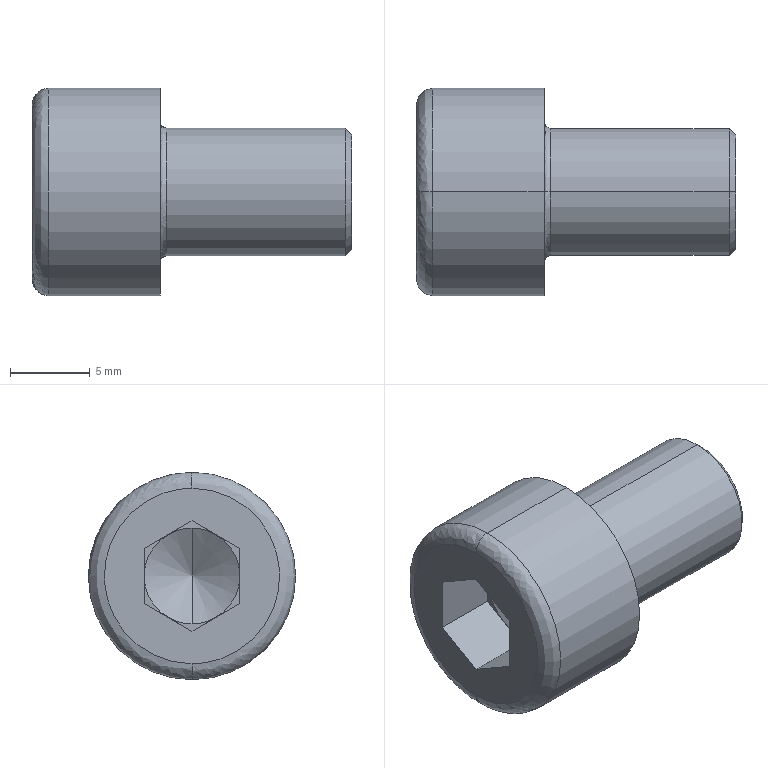Part | SolidWorks | features BaseBody 1 | 1 solid | 27 faces | box 20 x 13 x 13 mm | volume 1515 mm3 | plane 15 | spline 4 | cylinder 4 | cone 4 | commonest cylinder face diameters 8 x2 13 x2
STEP:
#1=CARTESIAN_POINT('',(1.,0.,6.5));
#2=VERTEX_POINT('',#1);
#3=CARTESIAN_POINT('',(1.,0.,-6.5));
#4=VERTEX_POINT('',#3);
#5=CARTESIAN_POINT('',(1.,0.,0.));
#6=DIRECTION('',(1.,0.,0.));
#7=DIRECTION('',(0.,0.,1.));
#8=AXIS2_PLACEMENT_3D('',#5,#6,#7);
#9=CIRCLE('',#8,6.5);
#10=EDGE_CURVE('',#2,#4,#9,.T.);
#11=ORIENTED_EDGE('',*,*,#10,.F.);
#12=CARTESIAN_POINT('',(0.,0.,5.5));
#13=VERTEX_POINT('',#12);
#14=CARTESIAN_POINT('',(1.,0.,5.5));
#15=DIRECTION('',(0.,-1.,0.));
#16=DIRECTION('',(0.,0.,1.));
#17=AXIS2_PLACEMENT_3D('',#14,#15,#16);
#18=CIRCLE('',#17,1.);
#19=EDGE_CURVE('',#2,#13,#18,.T.);
#20=ORIENTED_EDGE('',*,*,#19,.T.);
#21=CARTESIAN_POINT('',(0.,0.,-5.5));
#22=VERTEX_POINT('',#21);
#23=CARTESIAN_POINT('',(0.,0.,5.5));
#24=CARTESIAN_POINT('',(0.,-11.,5.5));
#25=CARTESIAN_POINT('',(0.,-11.,-5.5));
#26=CARTESIAN_POINT('',(0.,0.,-5.5));
#27=(BOUNDED_CURVE()B_SPLINE_CURVE(3,(#23,#24,#25,#26),.UNSPECIFIED.,.F.,.T.)B_SPLINE_CURVE_WITH_KNOTS((4,4),(0.,1.),.UNSPECIFIED.)CURVE()GEOMETRIC_REPRESENTATION_ITEM()RATIONAL_B_SPLINE_CURVE((1.,0.3333,0.3333,1.))REPRESENTATION_ITEM(''));
#28=EDGE_CURVE('',#13,#22,#27,.T.);
#29=ORIENTED_EDGE('',*,*,#28,.T.);
#30=CARTESIAN_POINT('',(1.,0.,-5.5));
#31=DIRECTION('',(0.,1.,0.));
#32=DIRECTION('',(0.,0.,-1.));
#33=AXIS2_PLACEMENT_3D('',#30,#31,#32);
#34=CIRCLE('',#33,1.);
#35=EDGE_CURVE('',#4,#22,#34,.T.);
#36=ORIENTED_EDGE('',*,*,#35,.F.);
#37=EDGE_LOOP('',(#11,#20,#29,#36));
#38=FACE_OUTER_BOUND('',#37,.T.);
#39=CARTESIAN_POINT('',(1.,0.,6.5));
#40=CARTESIAN_POINT('',(1.,-13.,6.5));
#41=CARTESIAN_POINT('',(1.,-13.,-6.5));
#42=CARTESIAN_POINT('',(1.,0.,-6.5));
#43=CARTESIAN_POINT('',(0.4142,0.,6.5));
#44=CARTESIAN_POINT('',(0.4142,-13.,6.5));
#45=CARTESIAN_POINT('',(0.4142,-13.,-6.5));
#46=CARTESIAN_POINT('',(0.4142,0.,-6.5));
#47=CARTESIAN_POINT('',(0.,0.,6.086));
#48=CARTESIAN_POINT('',(0.,-12.172,6.086));
#49=CARTESIAN_POINT('',(0.,-12.172,-6.086));
#50=CARTESIAN_POINT('',(0.,0.,-6.086));
#51=CARTESIAN_POINT('',(0.,0.,5.5));
#52=CARTESIAN_POINT('',(0.,-11.,5.5));
#53=CARTESIAN_POINT('',(0.,-11.,-5.5));
#54=CARTESIAN_POINT('',(0.,0.,-5.5));
#55=(BOUNDED_SURFACE()B_SPLINE_SURFACE(3,3,((#39,#40,#41,#42),(#43,#44,#45,#46),(#47,#48,#49,#50),(#51,#52,#53,#54)),.UNSPECIFIED.,.F.,.F.,.F.)B_SPLINE_SURFACE_WITH_KNOTS((4,4),(4,4),(0.,1.),(0.,1.),.UNSPECIFIED.)GEOMETRIC_REPRESENTATION_ITEM()RATIONAL_B_SPLINE_SURFACE(((1.,0.3333,0.3333,1.),(0.8047,0.2682,0.2682,0.8047),(0.8047,0.2682,0.2682,0.8047),(1.,0.3333,0.3333,1.)))REPRESENTATION_ITEM('')SURFACE());
#56=ADVANCED_FACE('',(#38),#55,.T.);
#57=CARTESIAN_POINT('',(8.,0.,4.4));
#58=VERTEX_POINT('',#57);
#59=CARTESIAN_POINT('',(8.,0.,-4.4));
#60=VERTEX_POINT('',#59);
#61=CARTESIAN_POINT('',(8.,0.,4.4));
#62=CARTESIAN_POINT('',(8.,0.2797,4.4));
#63=CARTESIAN_POINT('',(8.,0.6919,4.361));
#64=CARTESIAN_POINT('',(8.,1.16,4.249));
#65=CARTESIAN_POINT('',(8.,1.391,4.176));
#66=CARTESIAN_POINT('',(8.,1.489,4.141));
#67=CARTESIAN_POINT('',(8.,1.554,4.116));
#68=CARTESIAN_POINT('',(8.,1.585,4.105));
#69=CARTESIAN_POINT('',(8.,1.758,4.036));
#70=CARTESIAN_POINT('',(8.,1.96,3.944));
#71=CARTESIAN_POINT('',(8.,2.154,3.837));
#72=CARTESIAN_POINT('',(8.,2.282,3.763));
#73=CARTESIAN_POINT('',(8.,2.344,3.724));
#74=CARTESIAN_POINT('',(8.,2.662,3.517));
#75=CARTESIAN_POINT('',(8.,2.897,3.326));
#76=CARTESIAN_POINT('',(8.,3.219,3.004));
#77=CARTESIAN_POINT('',(8.,3.37,2.836));
#78=CARTESIAN_POINT('',(8.,3.509,2.656));
#79=CARTESIAN_POINT('',(8.,3.598,2.534));
#80=CARTESIAN_POINT('',(8.,3.642,2.47));
#81=CARTESIAN_POINT('',(8.,3.764,2.283));
#82=CARTESIAN_POINT('',(8.,3.876,2.092));
#83=CARTESIAN_POINT('',(8.,3.989,1.859));
#84=CARTESIAN_POINT('',(8.,4.042,1.74));
#85=CARTESIAN_POINT('',(8.,4.063,1.689));
#86=CARTESIAN_POINT('',(8.,4.077,1.654));
#87=CARTESIAN_POINT('',(8.,4.085,1.636));
#88=CARTESIAN_POINT('',(8.,4.297,1.1));
#89=CARTESIAN_POINT('',(8.,4.4,0.5592));
#90=CARTESIAN_POINT('',(8.,4.4,-0.2796));
#91=CARTESIAN_POINT('',(8.,4.361,-0.6917));
#92=CARTESIAN_POINT('',(8.,4.249,-1.16));
#93=CARTESIAN_POINT('',(8.,4.176,-1.391));
#94=CARTESIAN_POINT('',(8.,4.141,-1.489));
#95=CARTESIAN_POINT('',(8.,4.116,-1.554));
#96=CARTESIAN_POINT('',(8.,4.105,-1.585));
#97=CARTESIAN_POINT('',(8.,4.036,-1.758));
#98=CARTESIAN_POINT('',(8.,3.944,-1.96));
#99=CARTESIAN_POINT('',(8.,3.837,-2.154));
#100=CARTESIAN_POINT('',(8.,3.763,-2.282));
#101=CARTESIAN_POINT('',(8.,3.724,-2.344));
#102=CARTESIAN_POINT('',(8.,3.517,-2.662));
#103=CARTESIAN_POINT('',(8.,3.326,-2.897));
#104=CARTESIAN_POINT('',(8.,3.004,-3.219));
#105=CARTESIAN_POINT('',(8.,2.836,-3.37));
#106=CARTESIAN_POINT('',(8.,2.656,-3.509));
#107=CARTESIAN_POINT('',(8.,2.534,-3.598));
#108=CARTESIAN_POINT('',(8.,2.47,-3.642));
#109=CARTESIAN_POINT('',(8.,2.283,-3.764));
#110=CARTESIAN_POINT('',(8.,2.092,-3.876));
#111=CARTESIAN_POINT('',(8.,1.859,-3.989));
#112=CARTESIAN_POINT('',(8.,1.74,-4.042));
#113=CARTESIAN_POINT('',(8.,1.689,-4.063));
#114=CARTESIAN_POINT('',(8.,1.654,-4.077));
#115=CARTESIAN_POINT('',(8.,1.636,-4.085));
#116=CARTESIAN_POINT('',(8.,1.1,-4.297));
#117=CARTESIAN_POINT('',(8.,0.5597,-4.4));
#118=CARTESIAN_POINT('',(8.,0.,-4.4));
#119=B_SPLINE_CURVE_WITH_KNOTS('',3,(#61,#62,#63,#64,#65,#66,#67,#68,#69,#70,#71,#72,#73,#74,#75,#76,#77,#78,#79,#80,#81,#82,#83,#84,#85,#86,#87,#88,#89,#90,#91,#92,#93,#94,#95,#96,#97,#98,#99,#100,#101,#102,#103,#104,#105,#106,#107,#108,#109,#110,#111,#112,#113,#114,#115,#116,#117,#118),.UNSPECIFIED.,.F.,.F.,(4,1,1,1,2,2,1,2,2,2,1,2,2,1,1,1,2,2,2,1,1,1,2,2,1,2,2,2,1,2,2,1,1,1,2,2,4),(0.,0.0625,0.09375,0.1094,0.1172,0.125,0.1562,0.1719,0.1875,0.25,0.2812,0.2969,0.3125,0.3437,0.3594,0.3672,0.3711,0.375,0.5,0.5625,0.5937,0.6094,0.6172,0.625,0.6562,0.6719,0.6875,0.75,0.7812,0.7969,0.8125,0.8437,0.8594,0.8672,0.8711,0.875,1.),.UNSPECIFIED.);
#120=EDGE_CURVE('',#58,#60,#119,.T.);
#121=ORIENTED_EDGE('',*,*,#120,.F.);
#122=CARTESIAN_POINT('',(8.4,0.,4.));
#123=VERTEX_POINT('',#122);
#124=CARTESIAN_POINT('',(8.4,0.,4.4));
#125=DIRECTION('',(0.,-1.,0.));
#126=DIRECTION('',(0.,0.,1.));
#127=AXIS2_PLACEMENT_3D('',#124,#125,#126);
#128=CIRCLE('',#127,0.4);
#129=EDGE_CURVE('',#58,#123,#128,.T.);
#130=ORIENTED_EDGE('',*,*,#129,.T.);
#131=CARTESIAN_POINT('',(8.4,0.,-4.));
#132=VERTEX_POINT('',#131);
#133=CARTESIAN_POINT('',(8.4,0.,0.));
#134=DIRECTION('',(1.,0.,0.));
#135=DIRECTION('',(0.,0.,-1.));
#136=AXIS2_PLACEMENT_3D('',#133,#134,#135);
#137=CIRCLE('',#136,4.);
#138=EDGE_CURVE('',#132,#123,#137,.T.);
#139=ORIENTED_EDGE('',*,*,#138,.F.);
#140=CARTESIAN_POINT('',(8.4,0.,-4.4));
#141=DIRECTION('',(0.,1.,0.));
#142=DIRECTION('',(0.,0.,-1.));
#143=AXIS2_PLACEMENT_3D('',#140,#141,#142);
#144=CIRCLE('',#143,0.4);
#145=EDGE_CURVE('',#60,#132,#144,.T.);
#146=ORIENTED_EDGE('',*,*,#145,.F.);
#147=EDGE_LOOP('',(#121,#130,#139,#146));
#148=FACE_OUTER_BOUND('',#147,.T.);
#149=CARTESIAN_POINT('',(8.,0.,-4.4));
#150=CARTESIAN_POINT('',(8.,8.8,-4.4));
#151=CARTESIAN_POINT('',(8.,8.8,4.4));
#152=CARTESIAN_POINT('',(8.,0.,4.4));
#153=CARTESIAN_POINT('',(8.,0.,-4.166));
#154=CARTESIAN_POINT('',(8.,8.331,-4.166));
#155=CARTESIAN_POINT('',(8.,8.331,4.166));
#156=CARTESIAN_POINT('',(8.,0.,4.166));
#157=CARTESIAN_POINT('',(8.166,0.,-4.));
#158=CARTESIAN_POINT('',(8.166,8.,-4.));
#159=CARTESIAN_POINT('',(8.166,8.,4.));
#160=CARTESIAN_POINT('',(8.166,0.,4.));
#161=CARTESIAN_POINT('',(8.4,0.,-4.));
#162=CARTESIAN_POINT('',(8.4,8.,-4.));
#163=CARTESIAN_POINT('',(8.4,8.,4.));
#164=CARTESIAN_POINT('',(8.4,0.,4.));
#165=(BOUNDED_SURFACE()B_SPLINE_SURFACE(3,3,((#149,#150,#151,#152),(#153,#154,#155,#156),(#157,#158,#159,#160),(#161,#162,#163,#164)),.UNSPECIFIED.,.F.,.F.,.T.)B_SPLINE_SURFACE_WITH_KNOTS((4,4),(4,4),(0.,1.),(0.,1.),.UNSPECIFIED.)GEOMETRIC_REPRESENTATION_ITEM()RATIONAL_B_SPLINE_SURFACE(((1.,0.3333,0.3333,1.),(0.8047,0.2682,0.2682,0.8047),(0.8047,0.2682,0.2682,0.8047),(1.,0.3333,0.3333,1.)))REPRESENTATION_ITEM('')SURFACE());
#166=ADVANCED_FACE('',(#148),#165,.F.);
#167=CARTESIAN_POINT('',(8.,0.,6.5));
#168=VERTEX_POINT('',#167);
#169=CARTESIAN_POINT('',(8.,0.,-6.5));
#170=VERTEX_POINT('',#169);
#171=CARTESIAN_POINT('',(8.,0.,0.));
#172=DIRECTION('',(-1.,0.,0.));
#173=DIRECTION('',(0.,0.,1.));
#174=AXIS2_PLACEMENT_3D('',#171,#172,#173);
#175=CIRCLE('',#174,6.5);
#176=EDGE_CURVE('',#168,#170,#175,.T.);
#177=ORIENTED_EDGE('',*,*,#176,.T.);
#178=CARTESIAN_POINT('',(8.,0.,-6.5));
#179=DIRECTION('',(-1.,0.,0.));
#180=VECTOR('',#179,1000.);
#181=LINE('',#178,#180);
#182=EDGE_CURVE('',#170,#4,#181,.T.);
#183=ORIENTED_EDGE('',*,*,#182,.T.);
#184=CARTESIAN_POINT('',(1.,0.,0.));
#185=DIRECTION('',(1.,0.,0.));
#186=DIRECTION('',(0.,0.,1.));
#187=AXIS2_PLACEMENT_3D('',#184,#185,#186);
#188=CIRCLE('',#187,6.5);
#189=EDGE_CURVE('',#4,#2,#188,.T.);
#190=ORIENTED_EDGE('',*,*,#189,.T.);
#191=CARTESIAN_POINT('',(8.,0.,6.5));
#192=DIRECTION('',(-1.,0.,0.));
#193=VECTOR('',#192,1000.);
#194=LINE('',#191,#193);
#195=EDGE_CURVE('',#168,#2,#194,.T.);
#196=ORIENTED_EDGE('',*,*,#195,.F.);
#197=EDGE_LOOP('',(#177,#183,#190,#196));
#198=FACE_OUTER_BOUND('',#197,.T.);
#199=CARTESIAN_POINT('',(8.,0.,0.));
#200=DIRECTION('',(-1.,0.,0.));
#201=DIRECTION('',(0.,0.,1.));
#202=AXIS2_PLACEMENT_3D('',#199,#200,#201);
#203=CYLINDRICAL_SURFACE('',#202,6.5);
#204=ADVANCED_FACE('',(#198),#203,.T.);
#205=CARTESIAN_POINT('',(19.6,0.,4.));
#206=VERTEX_POINT('',#205);
#207=CARTESIAN_POINT('',(19.6,0.,-4.));
#208=VERTEX_POINT('',#207);
#209=CARTESIAN_POINT('',(19.6,0.,0.));
#210=DIRECTION('',(-1.,0.,0.));
#211=DIRECTION('',(0.,0.,1.));
#212=AXIS2_PLACEMENT_3D('',#209,#210,#211);
#213=CIRCLE('',#212,4.);
#214=EDGE_CURVE('',#206,#208,#213,.T.);
#215=ORIENTED_EDGE('',*,*,#214,.T.);
#216=CARTESIAN_POINT('',(20.,0.,-4.));
#217=DIRECTION('',(-1.,0.,0.));
#218=VECTOR('',#217,1000.);
#219=LINE('',#216,#218);
#220=EDGE_CURVE('',#208,#132,#219,.T.);
#221=ORIENTED_EDGE('',*,*,#220,.T.);
#222=ORIENTED_EDGE('',*,*,#138,.T.);
#223=CARTESIAN_POINT('',(20.,0.,4.));
#224=DIRECTION('',(-1.,0.,0.));
#225=VECTOR('',#224,1000.);
#226=LINE('',#223,#225);
#227=EDGE_CURVE('',#206,#123,#226,.T.);
#228=ORIENTED_EDGE('',*,*,#227,.F.);
#229=EDGE_LOOP('',(#215,#221,#222,#228));
#230=FACE_OUTER_BOUND('',#229,.T.);
#231=CARTESIAN_POINT('',(20.,0.,0.));
#232=DIRECTION('',(-1.,0.,0.));
#233=DIRECTION('',(0.,0.,1.));
#234=AXIS2_PLACEMENT_3D('',#231,#232,#233);
#235=CYLINDRICAL_SURFACE('',#234,4.);
#236=ADVANCED_FACE('',(#230),#235,.T.);
#237=CARTESIAN_POINT('',(20.,0.,3.6));
#238=VERTEX_POINT('',#237);
#239=CARTESIAN_POINT('',(20.,0.,-3.6));
#240=VERTEX_POINT('',#239);
#241=CARTESIAN_POINT('',(20.,0.,0.));
#242=DIRECTION('',(-1.,0.,0.));
#243=DIRECTION('',(0.,0.,1.));
#244=AXIS2_PLACEMENT_3D('',#241,#242,#243);
#245=CIRCLE('',#244,3.6);
#246=EDGE_CURVE('',#238,#240,#245,.T.);
#247=ORIENTED_EDGE('',*,*,#246,.T.);
#248=CARTESIAN_POINT('',(19.6,0.,-4.));
#249=DIRECTION('',(-0.7071,0.,-0.7071));
#250=VECTOR('',#249,1000.);
#251=LINE('',#248,#250);
#252=EDGE_CURVE('',#240,#208,#251,.T.);
#253=ORIENTED_EDGE('',*,*,#252,.T.);
#254=ORIENTED_EDGE('',*,*,#214,.F.);
#255=CARTESIAN_POINT('',(19.6,0.,4.));
#256=DIRECTION('',(-0.7071,0.,0.7071));
#257=VECTOR('',#256,1000.);
#258=LINE('',#255,#257);
#259=EDGE_CURVE('',#238,#206,#258,.T.);
#260=ORIENTED_EDGE('',*,*,#259,.F.);
#261=EDGE_LOOP('',(#247,#253,#254,#260));
#262=FACE_OUTER_BOUND('',#261,.T.);
#263=CARTESIAN_POINT('',(19.6,0.,0.));
#264=DIRECTION('',(-1.,0.,0.));
#265=DIRECTION('',(0.,0.,1.));
#266=AXIS2_PLACEMENT_3D('',#263,#264,#265);
#267=CONICAL_SURFACE('',#266,4.,0.7854);
#268=ADVANCED_FACE('',(#262),#267,.T.);
#269=CARTESIAN_POINT('',(5.732,0.,0.));
#270=VERTEX_POINT('',#269);
#271=CARTESIAN_POINT('',(4.,0.,3.));
#272=VERTEX_POINT('',#271);
#273=CARTESIAN_POINT('',(4.,0.,3.));
#274=DIRECTION('',(-0.5,0.,0.866));
#275=VECTOR('',#274,1000.);
#276=LINE('',#273,#275);
#277=EDGE_CURVE('',#270,#272,#276,.T.);
#278=ORIENTED_EDGE('',*,*,#277,.F.);
#279=CARTESIAN_POINT('',(4.,0.,-3.));
#280=VERTEX_POINT('',#279);
#281=CARTESIAN_POINT('',(4.,0.,-3.));
#282=DIRECTION('',(-0.5,0.,-0.866));
#283=VECTOR('',#282,1000.);
#284=LINE('',#281,#283);
#285=EDGE_CURVE('',#270,#280,#284,.T.);
#286=ORIENTED_EDGE('',*,*,#285,.T.);
#287=CARTESIAN_POINT('',(4.,-1.5,-2.598));
#288=VERTEX_POINT('',#287);
#289=CARTESIAN_POINT('',(4.,0.,0.));
#290=DIRECTION('',(1.,0.,0.));
#291=DIRECTION('',(0.,0.,1.));
#292=AXIS2_PLACEMENT_3D('',#289,#290,#291);
#293=CIRCLE('',#292,3.);
#294=EDGE_CURVE('',#288,#280,#293,.T.);
#295=ORIENTED_EDGE('',*,*,#294,.F.);
#296=CARTESIAN_POINT('',(4.,-3.,0.));
#297=VERTEX_POINT('',#296);
#298=CARTESIAN_POINT('',(4.,0.,0.));
#299=DIRECTION('',(-1.,0.,0.));
#300=DIRECTION('',(0.,0.,1.));
#301=AXIS2_PLACEMENT_3D('',#298,#299,#300);
#302=CIRCLE('',#301,3.);
#303=EDGE_CURVE('',#288,#297,#302,.T.);
#304=ORIENTED_EDGE('',*,*,#303,.T.);
#305=CARTESIAN_POINT('',(4.,-1.5,2.598));
#306=VERTEX_POINT('',#305);
#307=CARTESIAN_POINT('',(4.,0.,0.));
#308=DIRECTION('',(1.,0.,0.));
#309=DIRECTION('',(0.,0.,1.));
#310=AXIS2_PLACEMENT_3D('',#307,#308,#309);
#311=CIRCLE('',#310,3.);
#312=EDGE_CURVE('',#306,#297,#311,.T.);
#313=ORIENTED_EDGE('',*,*,#312,.F.);
#314=CARTESIAN_POINT('',(4.,0.,0.));
#315=DIRECTION('',(1.,0.,0.));
#316=DIRECTION('',(0.,0.,1.));
#317=AXIS2_PLACEMENT_3D('',#314,#315,#316);
#318=CIRCLE('',#317,3.);
#319=EDGE_CURVE('',#272,#306,#318,.T.);
#320=ORIENTED_EDGE('',*,*,#319,.F.);
#321=EDGE_LOOP('',(#278,#286,#295,#304,#313,#320));
#322=FACE_OUTER_BOUND('',#321,.T.);
#323=CARTESIAN_POINT('',(4.,0.,0.));
#324=DIRECTION('',(-1.,0.,0.));
#325=DIRECTION('',(0.,0.,1.));
#326=AXIS2_PLACEMENT_3D('',#323,#324,#325);
#327=CONICAL_SURFACE('',#326,3.,1.047);
#328=ADVANCED_FACE('',(#322),#327,.F.);
#329=ORIENTED_EDGE('',*,*,#182,.F.);
#330=CARTESIAN_POINT('',(8.,0.,0.));
#331=DIRECTION('',(-1.,0.,0.));
#332=DIRECTION('',(0.,0.,1.));
#333=AXIS2_PLACEMENT_3D('',#330,#331,#332);
#334=CIRCLE('',#333,6.5);
#335=EDGE_CURVE('',#170,#168,#334,.T.);
#336=ORIENTED_EDGE('',*,*,#335,.T.);
#337=ORIENTED_EDGE('',*,*,#195,.T.);
#338=ORIENTED_EDGE('',*,*,#10,.T.);
#339=EDGE_LOOP('',(#329,#336,#337,#338));
#340=FACE_OUTER_BOUND('',#339,.T.);
#341=CARTESIAN_POINT('',(8.,0.,0.));
#342=DIRECTION('',(-1.,0.,0.));
#343=DIRECTION('',(0.,0.,1.));
#344=AXIS2_PLACEMENT_3D('',#341,#342,#343);
#345=CYLINDRICAL_SURFACE('',#344,6.5);
#346=ADVANCED_FACE('',(#340),#345,.T.);
#347=ORIENTED_EDGE('',*,*,#19,.F.);
#348=ORIENTED_EDGE('',*,*,#189,.F.);
#349=ORIENTED_EDGE('',*,*,#35,.T.);
#350=CARTESIAN_POINT('',(0.,0.,-5.5));
#351=CARTESIAN_POINT('',(0.,11.,-5.5));
#352=CARTESIAN_POINT('',(0.,11.,5.5));
#353=CARTESIAN_POINT('',(0.,0.,5.5));
#354=(BOUNDED_CURVE()B_SPLINE_CURVE(3,(#350,#351,#352,#353),.UNSPECIFIED.,.F.,.F.)B_SPLINE_CURVE_WITH_KNOTS((4,4),(0.,1.),.UNSPECIFIED.)CURVE()GEOMETRIC_REPRESENTATION_ITEM()RATIONAL_B_SPLINE_CURVE((1.,0.3333,0.3333,1.))REPRESENTATION_ITEM(''));
#355=EDGE_CURVE('',#22,#13,#354,.T.);
#356=ORIENTED_EDGE('',*,*,#355,.T.);
#357=EDGE_LOOP('',(#347,#348,#349,#356));
#358=FACE_OUTER_BOUND('',#357,.T.);
#359=CARTESIAN_POINT('',(1.,0.,-6.5));
#360=CARTESIAN_POINT('',(1.,13.,-6.5));
#361=CARTESIAN_POINT('',(1.,13.,6.5));
#362=CARTESIAN_POINT('',(1.,0.,6.5));
#363=CARTESIAN_POINT('',(0.4142,0.,-6.5));
#364=CARTESIAN_POINT('',(0.4142,13.,-6.5));
#365=CARTESIAN_POINT('',(0.4142,13.,6.5));
#366=CARTESIAN_POINT('',(0.4142,0.,6.5));
#367=CARTESIAN_POINT('',(0.,0.,-6.086));
#368=CARTESIAN_POINT('',(0.,12.172,-6.086));
#369=CARTESIAN_POINT('',(0.,12.172,6.086));
#370=CARTESIAN_POINT('',(0.,0.,6.086));
#371=CARTESIAN_POINT('',(0.,0.,-5.5));
#372=CARTESIAN_POINT('',(0.,11.,-5.5));
#373=CARTESIAN_POINT('',(0.,11.,5.5));
#374=CARTESIAN_POINT('',(0.,0.,5.5));
#375=(BOUNDED_SURFACE()B_SPLINE_SURFACE(3,3,((#359,#360,#361,#362),(#363,#364,#365,#366),(#367,#368,#369,#370),(#371,#372,#373,#374)),.UNSPECIFIED.,.F.,.F.,.T.)B_SPLINE_SURFACE_WITH_KNOTS((4,4),(4,4),(0.,1.),(0.,1.),.UNSPECIFIED.)GEOMETRIC_REPRESENTATION_ITEM()RATIONAL_B_SPLINE_SURFACE(((1.,0.3333,0.3333,1.),(0.8047,0.2682,0.2682,0.8047),(0.8047,0.2682,0.2682,0.8047),(1.,0.3333,0.3333,1.)))REPRESENTATION_ITEM('')SURFACE());
#376=ADVANCED_FACE('',(#358),#375,.T.);
#377=ORIENTED_EDGE('',*,*,#176,.F.);
#378=ORIENTED_EDGE('',*,*,#335,.F.);
#379=EDGE_LOOP('',(#377,#378));
#380=FACE_OUTER_BOUND('',#379,.T.);
#381=CARTESIAN_POINT('',(8.,0.,-4.4));
#382=CARTESIAN_POINT('',(8.,-0.2797,-4.4));
#383=CARTESIAN_POINT('',(8.,-0.6919,-4.361));
#384=CARTESIAN_POINT('',(8.,-1.16,-4.249));
#385=CARTESIAN_POINT('',(8.,-1.391,-4.176));
#386=CARTESIAN_POINT('',(8.,-1.489,-4.141));
#387=CARTESIAN_POINT('',(8.,-1.554,-4.116));
#388=CARTESIAN_POINT('',(8.,-1.585,-4.105));
#389=CARTESIAN_POINT('',(8.,-1.758,-4.036));
#390=CARTESIAN_POINT('',(8.,-1.96,-3.944));
#391=CARTESIAN_POINT('',(8.,-2.154,-3.837));
#392=CARTESIAN_POINT('',(8.,-2.282,-3.763));
#393=CARTESIAN_POINT('',(8.,-2.344,-3.724));
#394=CARTESIAN_POINT('',(8.,-2.662,-3.517));
#395=CARTESIAN_POINT('',(8.,-2.897,-3.326));
#396=CARTESIAN_POINT('',(8.,-3.219,-3.004));
#397=CARTESIAN_POINT('',(8.,-3.37,-2.836));
#398=CARTESIAN_POINT('',(8.,-3.509,-2.656));
#399=CARTESIAN_POINT('',(8.,-3.598,-2.534));
#400=CARTESIAN_POINT('',(8.,-3.642,-2.47));
#401=CARTESIAN_POINT('',(8.,-3.764,-2.283));
#402=CARTESIAN_POINT('',(8.,-3.876,-2.092));
#403=CARTESIAN_POINT('',(8.,-3.989,-1.859));
#404=CARTESIAN_POINT('',(8.,-4.042,-1.74));
#405=CARTESIAN_POINT('',(8.,-4.063,-1.689));
#406=CARTESIAN_POINT('',(8.,-4.077,-1.654));
#407=CARTESIAN_POINT('',(8.,-4.085,-1.636));
#408=CARTESIAN_POINT('',(8.,-4.297,-1.1));
#409=CARTESIAN_POINT('',(8.,-4.4,-0.5592));
#410=CARTESIAN_POINT('',(8.,-4.4,0.2796));
#411=CARTESIAN_POINT('',(8.,-4.361,0.6917));
#412=CARTESIAN_POINT('',(8.,-4.249,1.16));
#413=CARTESIAN_POINT('',(8.,-4.176,1.391));
#414=CARTESIAN_POINT('',(8.,-4.141,1.489));
#415=CARTESIAN_POINT('',(8.,-4.116,1.554));
#416=CARTESIAN_POINT('',(8.,-4.105,1.585));
#417=CARTESIAN_POINT('',(8.,-4.036,1.758));
#418=CARTESIAN_POINT('',(8.,-3.944,1.96));
#419=CARTESIAN_POINT('',(8.,-3.837,2.154));
#420=CARTESIAN_POINT('',(8.,-3.763,2.282));
#421=CARTESIAN_POINT('',(8.,-3.724,2.344));
#422=CARTESIAN_POINT('',(8.,-3.517,2.662));
#423=CARTESIAN_POINT('',(8.,-3.326,2.897));
#424=CARTESIAN_POINT('',(8.,-3.004,3.219));
#425=CARTESIAN_POINT('',(8.,-2.836,3.37));
#426=CARTESIAN_POINT('',(8.,-2.656,3.509));
#427=CARTESIAN_POINT('',(8.,-2.534,3.598));
#428=CARTESIAN_POINT('',(8.,-2.47,3.642));
#429=CARTESIAN_POINT('',(8.,-2.283,3.764));
#430=CARTESIAN_POINT('',(8.,-2.092,3.876));
#431=CARTESIAN_POINT('',(8.,-1.859,3.989));
#432=CARTESIAN_POINT('',(8.,-1.74,4.042));
#433=CARTESIAN_POINT('',(8.,-1.689,4.063));
#434=CARTESIAN_POINT('',(8.,-1.654,4.077));
#435=CARTESIAN_POINT('',(8.,-1.636,4.085));
#436=CARTESIAN_POINT('',(8.,-1.1,4.297));
#437=CARTESIAN_POINT('',(8.,-0.5597,4.4));
#438=CARTESIAN_POINT('',(8.,0.,4.4));
#439=B_SPLINE_CURVE_WITH_KNOTS('',3,(#381,#382,#383,#384,#385,#386,#387,#388,#389,#390,#391,#392,#393,#394,#395,#396,#397,#398,#399,#400,#401,#402,#403,#404,#405,#406,#407,#408,#409,#410,#411,#412,#413,#414,#415,#416,#417,#418,#419,#420,#421,#422,#423,#424,#425,#426,#427,#428,#429,#430,#431,#432,#433,#434,#435,#436,#437,#438),.UNSPECIFIED.,.F.,.F.,(4,1,1,1,2,2,1,2,2,2,1,2,2,1,1,1,2,2,2,1,1,1,2,2,1,2,2,2,1,2,2,1,1,1,2,2,4),(0.,0.0625,0.09375,0.1094,0.1172,0.125,0.1563,0.1719,0.1875,0.25,0.2813,0.2969,0.3125,0.3438,0.3594,0.3672,0.3711,0.375,0.5,0.5625,0.5938,0.6094,0.6172,0.625,0.6563,0.6719,0.6875,0.75,0.7813,0.7969,0.8125,0.8438,0.8594,0.8672,0.8711,0.875,1.),.UNSPECIFIED.);
#440=EDGE_CURVE('',#60,#58,#439,.T.);
#441=ORIENTED_EDGE('',*,*,#440,.T.);
#442=ORIENTED_EDGE('',*,*,#120,.T.);
#443=EDGE_LOOP('',(#441,#442));
#444=FACE_BOUND('',#443,.T.);
#445=CARTESIAN_POINT('',(8.,0.,0.));
#446=DIRECTION('',(1.,0.,0.));
#447=DIRECTION('',(0.,0.,-1.));
#448=AXIS2_PLACEMENT_3D('',#445,#446,#447);
#449=PLANE('',#448);
#450=ADVANCED_FACE('',(#380,#444),#449,.T.);
#451=CARTESIAN_POINT('',(0.,3.,1.732));
#452=VERTEX_POINT('',#451);
#453=CARTESIAN_POINT('',(0.,3.,-1.732));
#454=VERTEX_POINT('',#453);
#455=CARTESIAN_POINT('',(0.,3.,0.));
#456=DIRECTION('',(0.,0.,-1.));
#457=VECTOR('',#456,1000.);
#458=LINE('',#455,#457);
#459=EDGE_CURVE('',#452,#454,#458,.T.);
#460=ORIENTED_EDGE('',*,*,#459,.F.);
#461=CARTESIAN_POINT('',(0.,0.,3.464));
#462=VERTEX_POINT('',#461);
#463=CARTESIAN_POINT('',(0.,0.,3.464));
#464=DIRECTION('',(0.,0.866,-0.5));
#465=VECTOR('',#464,1000.);
#466=LINE('',#463,#465);
#467=EDGE_CURVE('',#462,#452,#466,.T.);
#468=ORIENTED_EDGE('',*,*,#467,.F.);
#469=CARTESIAN_POINT('',(0.,-3.,1.732));
#470=VERTEX_POINT('',#469);
#471=CARTESIAN_POINT('',(0.,-3.,1.732));
#472=DIRECTION('',(0.,0.866,0.5));
#473=VECTOR('',#472,1000.);
#474=LINE('',#471,#473);
#475=EDGE_CURVE('',#470,#462,#474,.T.);
#476=ORIENTED_EDGE('',*,*,#475,.F.);
#477=CARTESIAN_POINT('',(0.,-3.,-1.732));
#478=VERTEX_POINT('',#477);
#479=CARTESIAN_POINT('',(0.,-3.,0.));
#480=DIRECTION('',(0.,0.,1.));
#481=VECTOR('',#480,1000.);
#482=LINE('',#479,#481);
#483=EDGE_CURVE('',#478,#470,#482,.T.);
#484=ORIENTED_EDGE('',*,*,#483,.F.);
#485=CARTESIAN_POINT('',(0.,0.,-3.464));
#486=VERTEX_POINT('',#485);
#487=CARTESIAN_POINT('',(0.,0.,-3.464));
#488=DIRECTION('',(0.,-0.866,0.5));
#489=VECTOR('',#488,1000.);
#490=LINE('',#487,#489);
#491=EDGE_CURVE('',#486,#478,#490,.T.);
#492=ORIENTED_EDGE('',*,*,#491,.F.);
#493=CARTESIAN_POINT('',(0.,3.,-1.732));
#494=DIRECTION('',(0.,-0.866,-0.5));
#495=VECTOR('',#494,1000.);
#496=LINE('',#493,#495);
#497=EDGE_CURVE('',#454,#486,#496,.T.);
#498=ORIENTED_EDGE('',*,*,#497,.F.);
#499=EDGE_LOOP('',(#460,#468,#476,#484,#492,#498));
#500=FACE_BOUND('',#499,.T.);
#501=ORIENTED_EDGE('',*,*,#355,.F.);
#502=ORIENTED_EDGE('',*,*,#28,.F.);
#503=EDGE_LOOP('',(#501,#502));
#504=FACE_OUTER_BOUND('',#503,.T.);
#505=CARTESIAN_POINT('',(0.,0.,0.));
#506=DIRECTION('',(1.,0.,0.));
#507=DIRECTION('',(0.,0.,-1.));
#508=AXIS2_PLACEMENT_3D('',#505,#506,#507);
#509=PLANE('',#508);
#510=ADVANCED_FACE('',(#500,#504),#509,.F.);
#511=ORIENTED_EDGE('',*,*,#129,.F.);
#512=ORIENTED_EDGE('',*,*,#440,.F.);
#513=ORIENTED_EDGE('',*,*,#145,.T.);
#514=CARTESIAN_POINT('',(8.4,0.,0.));
#515=DIRECTION('',(1.,0.,0.));
#516=DIRECTION('',(0.,0.,-1.));
#517=AXIS2_PLACEMENT_3D('',#514,#515,#516);
#518=CIRCLE('',#517,4.);
#519=EDGE_CURVE('',#123,#132,#518,.T.);
#520=ORIENTED_EDGE('',*,*,#519,.F.);
#521=EDGE_LOOP('',(#511,#512,#513,#520));
#522=FACE_OUTER_BOUND('',#521,.T.);
#523=CARTESIAN_POINT('',(8.,0.,4.4));
#524=CARTESIAN_POINT('',(8.,-8.8,4.4));
#525=CARTESIAN_POINT('',(8.,-8.8,-4.4));
#526=CARTESIAN_POINT('',(8.,0.,-4.4));
#527=CARTESIAN_POINT('',(8.,0.,4.166));
#528=CARTESIAN_POINT('',(8.,-8.331,4.166));
#529=CARTESIAN_POINT('',(8.,-8.331,-4.166));
#530=CARTESIAN_POINT('',(8.,0.,-4.166));
#531=CARTESIAN_POINT('',(8.166,0.,4.));
#532=CARTESIAN_POINT('',(8.166,-8.,4.));
#533=CARTESIAN_POINT('',(8.166,-8.,-4.));
#534=CARTESIAN_POINT('',(8.166,0.,-4.));
#535=CARTESIAN_POINT('',(8.4,0.,4.));
#536=CARTESIAN_POINT('',(8.4,-8.,4.));
#537=CARTESIAN_POINT('',(8.4,-8.,-4.));
#538=CARTESIAN_POINT('',(8.4,0.,-4.));
#539=(BOUNDED_SURFACE()B_SPLINE_SURFACE(3,3,((#523,#524,#525,#526),(#527,#528,#529,#530),(#531,#532,#533,#534),(#535,#536,#537,#538)),.UNSPECIFIED.,.F.,.F.,.T.)B_SPLINE_SURFACE_WITH_KNOTS((4,4),(4,4),(0.,1.),(0.,1.),.UNSPECIFIED.)GEOMETRIC_REPRESENTATION_ITEM()RATIONAL_B_SPLINE_SURFACE(((1.,0.3333,0.3333,1.),(0.8047,0.2682,0.2682,0.8047),(0.8047,0.2682,0.2682,0.8047),(1.,0.3333,0.3333,1.)))REPRESENTATION_ITEM('')SURFACE());
#540=ADVANCED_FACE('',(#522),#539,.F.);
#541=CARTESIAN_POINT('',(4.,0.,-3.464));
#542=VERTEX_POINT('',#541);
#543=CARTESIAN_POINT('',(4.,0.,-3.464));
#544=DIRECTION('',(1.,0.,0.));
#545=VECTOR('',#544,1000.);
#546=LINE('',#543,#545);
#547=EDGE_CURVE('',#486,#542,#546,.T.);
#548=ORIENTED_EDGE('',*,*,#547,.T.);
#549=CARTESIAN_POINT('',(4.,1.5,-2.598));
#550=VERTEX_POINT('',#549);
#551=CARTESIAN_POINT('',(4.,0.,-3.464));
#552=DIRECTION('',(0.,0.866,0.5));
#553=VECTOR('',#552,1000.);
#554=LINE('',#551,#553);
#555=EDGE_CURVE('',#542,#550,#554,.T.);
#556=ORIENTED_EDGE('',*,*,#555,.T.);
#557=CARTESIAN_POINT('',(4.,3.,-1.732));
#558=VERTEX_POINT('',#557);
#559=CARTESIAN_POINT('',(4.,1.5,-2.598));
#560=DIRECTION('',(0.,0.866,0.5));
#561=VECTOR('',#560,1000.);
#562=LINE('',#559,#561);
#563=EDGE_CURVE('',#550,#558,#562,.T.);
#564=ORIENTED_EDGE('',*,*,#563,.T.);
#565=CARTESIAN_POINT('',(4.,3.,-1.732));
#566=DIRECTION('',(-1.,0.,0.));
#567=VECTOR('',#566,1000.);
#568=LINE('',#565,#567);
#569=EDGE_CURVE('',#558,#454,#568,.T.);
#570=ORIENTED_EDGE('',*,*,#569,.T.);
#571=ORIENTED_EDGE('',*,*,#497,.T.);
#572=EDGE_LOOP('',(#548,#556,#564,#570,#571));
#573=FACE_OUTER_BOUND('',#572,.T.);
#574=CARTESIAN_POINT('',(4.,0.,-3.464));
#575=DIRECTION('',(0.,-0.5,0.866));
#576=DIRECTION('',(0.,-0.866,-0.5));
#577=AXIS2_PLACEMENT_3D('',#574,#575,#576);
#578=PLANE('',#577);
#579=ADVANCED_FACE('',(#573),#578,.T.);
#580=ORIENTED_EDGE('',*,*,#569,.F.);
#581=CARTESIAN_POINT('',(4.,3.,0.));
#582=VERTEX_POINT('',#581);
#583=CARTESIAN_POINT('',(4.,3.,-3.464));
#584=DIRECTION('',(0.,0.,1.));
#585=VECTOR('',#584,1000.);
#586=LINE('',#583,#585);
#587=EDGE_CURVE('',#558,#582,#586,.T.);
#588=ORIENTED_EDGE('',*,*,#587,.T.);
#589=CARTESIAN_POINT('',(4.,3.,1.732));
#590=VERTEX_POINT('',#589);
#591=CARTESIAN_POINT('',(4.,3.,-3.464));
#592=DIRECTION('',(0.,0.,1.));
#593=VECTOR('',#592,1000.);
#594=LINE('',#591,#593);
#595=EDGE_CURVE('',#582,#590,#594,.T.);
#596=ORIENTED_EDGE('',*,*,#595,.T.);
#597=CARTESIAN_POINT('',(4.,3.,1.732));
#598=DIRECTION('',(-1.,0.,0.));
#599=VECTOR('',#598,1000.);
#600=LINE('',#597,#599);
#601=EDGE_CURVE('',#590,#452,#600,.T.);
#602=ORIENTED_EDGE('',*,*,#601,.T.);
#603=ORIENTED_EDGE('',*,*,#459,.T.);
#604=EDGE_LOOP('',(#580,#588,#596,#602,#603));
#605=FACE_OUTER_BOUND('',#604,.T.);
#606=CARTESIAN_POINT('',(4.,3.,-1.732));
#607=DIRECTION('',(0.,-1.,0.));
#608=DIRECTION('',(0.,0.,-1.));
#609=AXIS2_PLACEMENT_3D('',#606,#607,#608);
#610=PLANE('',#609);
#611=ADVANCED_FACE('',(#605),#610,.T.);
#612=ORIENTED_EDGE('',*,*,#601,.F.);
#613=CARTESIAN_POINT('',(4.,1.5,2.598));
#614=VERTEX_POINT('',#613);
#615=CARTESIAN_POINT('',(4.,3.,1.732));
#616=DIRECTION('',(0.,-0.866,0.5));
#617=VECTOR('',#616,1000.);
#618=LINE('',#615,#617);
#619=EDGE_CURVE('',#590,#614,#618,.T.);
#620=ORIENTED_EDGE('',*,*,#619,.T.);
#621=CARTESIAN_POINT('',(4.,0.,3.464));
#622=VERTEX_POINT('',#621);
#623=CARTESIAN_POINT('',(4.,3.,1.732));
#624=DIRECTION('',(0.,-0.866,0.5));
#625=VECTOR('',#624,1000.);
#626=LINE('',#623,#625);
#627=EDGE_CURVE('',#614,#622,#626,.T.);
#628=ORIENTED_EDGE('',*,*,#627,.T.);
#629=CARTESIAN_POINT('',(4.,0.,3.464));
#630=DIRECTION('',(-1.,0.,0.));
#631=VECTOR('',#630,1000.);
#632=LINE('',#629,#631);
#633=EDGE_CURVE('',#622,#462,#632,.T.);
#634=ORIENTED_EDGE('',*,*,#633,.T.);
#635=ORIENTED_EDGE('',*,*,#467,.T.);
#636=EDGE_LOOP('',(#612,#620,#628,#634,#635));
#637=FACE_OUTER_BOUND('',#636,.T.);
#638=CARTESIAN_POINT('',(4.,3.,1.732));
#639=DIRECTION('',(0.,-0.5,-0.866));
#640=DIRECTION('',(0.,0.866,-0.5));
#641=AXIS2_PLACEMENT_3D('',#638,#639,#640);
#642=PLANE('',#641);
#643=ADVANCED_FACE('',(#637),#642,.T.);
#644=ORIENTED_EDGE('',*,*,#633,.F.);
#645=CARTESIAN_POINT('',(4.,0.,3.464));
#646=DIRECTION('',(0.,-0.866,-0.5));
#647=VECTOR('',#646,1000.);
#648=LINE('',#645,#647);
#649=EDGE_CURVE('',#622,#306,#648,.T.);
#650=ORIENTED_EDGE('',*,*,#649,.T.);
#651=CARTESIAN_POINT('',(4.,-3.,1.732));
#652=VERTEX_POINT('',#651);
#653=CARTESIAN_POINT('',(4.,-1.5,2.598));
#654=DIRECTION('',(0.,-0.866,-0.5));
#655=VECTOR('',#654,1000.);
#656=LINE('',#653,#655);
#657=EDGE_CURVE('',#306,#652,#656,.T.);
#658=ORIENTED_EDGE('',*,*,#657,.T.);
#659=CARTESIAN_POINT('',(4.,-3.,1.732));
#660=DIRECTION('',(-1.,0.,0.));
#661=VECTOR('',#660,1000.);
#662=LINE('',#659,#661);
#663=EDGE_CURVE('',#652,#470,#662,.T.);
#664=ORIENTED_EDGE('',*,*,#663,.T.);
#665=ORIENTED_EDGE('',*,*,#475,.T.);
#666=EDGE_LOOP('',(#644,#650,#658,#664,#665));
#667=FACE_OUTER_BOUND('',#666,.T.);
#668=CARTESIAN_POINT('',(4.,0.,3.464));
#669=DIRECTION('',(0.,0.5,-0.866));
#670=DIRECTION('',(0.,0.866,0.5));
#671=AXIS2_PLACEMENT_3D('',#668,#669,#670);
#672=PLANE('',#671);
#673=ADVANCED_FACE('',(#667),#672,.T.);
#674=ORIENTED_EDGE('',*,*,#663,.F.);
#675=CARTESIAN_POINT('',(4.,-3.,-3.464));
#676=DIRECTION('',(0.,0.,-1.));
#677=VECTOR('',#676,1000.);
#678=LINE('',#675,#677);
#679=EDGE_CURVE('',#652,#297,#678,.T.);
#680=ORIENTED_EDGE('',*,*,#679,.T.);
#681=CARTESIAN_POINT('',(4.,-3.,-1.732));
#682=VERTEX_POINT('',#681);
#683=CARTESIAN_POINT('',(4.,-3.,1.732));
#684=DIRECTION('',(0.,0.,-1.));
#685=VECTOR('',#684,1000.);
#686=LINE('',#683,#685);
#687=EDGE_CURVE('',#297,#682,#686,.T.);
#688=ORIENTED_EDGE('',*,*,#687,.T.);
#689=CARTESIAN_POINT('',(4.,-3.,-1.732));
#690=DIRECTION('',(-1.,0.,0.));
#691=VECTOR('',#690,1000.);
#692=LINE('',#689,#691);
#693=EDGE_CURVE('',#682,#478,#692,.T.);
#694=ORIENTED_EDGE('',*,*,#693,.T.);
#695=ORIENTED_EDGE('',*,*,#483,.T.);
#696=EDGE_LOOP('',(#674,#680,#688,#694,#695));
#697=FACE_OUTER_BOUND('',#696,.T.);
#698=CARTESIAN_POINT('',(4.,-3.,1.732));
#699=DIRECTION('',(0.,1.,0.));
#700=DIRECTION('',(0.,0.,1.));
#701=AXIS2_PLACEMENT_3D('',#698,#699,#700);
#702=PLANE('',#701);
#703=ADVANCED_FACE('',(#697),#702,.T.);
#704=ORIENTED_EDGE('',*,*,#693,.F.);
#705=CARTESIAN_POINT('',(4.,-3.,-1.732));
#706=DIRECTION('',(0.,0.866,-0.5));
#707=VECTOR('',#706,1000.);
#708=LINE('',#705,#707);
#709=EDGE_CURVE('',#682,#288,#708,.T.);
#710=ORIENTED_EDGE('',*,*,#709,.T.);
#711=CARTESIAN_POINT('',(4.,-3.,-1.732));
#712=DIRECTION('',(0.,0.866,-0.5));
#713=VECTOR('',#712,1000.);
#714=LINE('',#711,#713);
#715=EDGE_CURVE('',#288,#542,#714,.T.);
#716=ORIENTED_EDGE('',*,*,#715,.T.);
#717=ORIENTED_EDGE('',*,*,#547,.F.);
#718=ORIENTED_EDGE('',*,*,#491,.T.);
#719=EDGE_LOOP('',(#704,#710,#716,#717,#718));
#720=FACE_OUTER_BOUND('',#719,.T.);
#721=CARTESIAN_POINT('',(4.,-3.,-1.732));
#722=DIRECTION('',(0.,0.5,0.866));
#723=DIRECTION('',(0.,-0.866,0.5));
#724=AXIS2_PLACEMENT_3D('',#721,#722,#723);
#725=PLANE('',#724);
#726=ADVANCED_FACE('',(#720),#725,.T.);
#727=ORIENTED_EDGE('',*,*,#220,.F.);
#728=CARTESIAN_POINT('',(19.6,0.,0.));
#729=DIRECTION('',(-1.,0.,0.));
#730=DIRECTION('',(0.,0.,1.));
#731=AXIS2_PLACEMENT_3D('',#728,#729,#730);
#732=CIRCLE('',#731,4.);
#733=EDGE_CURVE('',#208,#206,#732,.T.);
#734=ORIENTED_EDGE('',*,*,#733,.T.);
#735=ORIENTED_EDGE('',*,*,#227,.T.);
#736=ORIENTED_EDGE('',*,*,#519,.T.);
#737=EDGE_LOOP('',(#727,#734,#735,#736));
#738=FACE_OUTER_BOUND('',#737,.T.);
#739=CARTESIAN_POINT('',(20.,0.,0.));
#740=DIRECTION('',(-1.,0.,0.));
#741=DIRECTION('',(0.,0.,1.));
#742=AXIS2_PLACEMENT_3D('',#739,#740,#741);
#743=CYLINDRICAL_SURFACE('',#742,4.);
#744=ADVANCED_FACE('',(#738),#743,.T.);
#745=ORIENTED_EDGE('',*,*,#294,.T.);
#746=CARTESIAN_POINT('',(4.,0.,0.));
#747=DIRECTION('',(1.,0.,0.));
#748=DIRECTION('',(0.,0.,1.));
#749=AXIS2_PLACEMENT_3D('',#746,#747,#748);
#750=CIRCLE('',#749,3.);
#751=EDGE_CURVE('',#280,#550,#750,.T.);
#752=ORIENTED_EDGE('',*,*,#751,.T.);
#753=ORIENTED_EDGE('',*,*,#555,.F.);
#754=ORIENTED_EDGE('',*,*,#715,.F.);
#755=EDGE_LOOP('',(#745,#752,#753,#754));
#756=FACE_OUTER_BOUND('',#755,.T.);
#757=CARTESIAN_POINT('',(4.,0.,-3.464));
#758=DIRECTION('',(1.,0.,0.));
#759=DIRECTION('',(0.,0.,-1.));
#760=AXIS2_PLACEMENT_3D('',#757,#758,#759);
#761=PLANE('',#760);
#762=ADVANCED_FACE('',(#756),#761,.F.);
#763=ORIENTED_EDGE('',*,*,#627,.F.);
#764=CARTESIAN_POINT('',(4.,0.,0.));
#765=DIRECTION('',(1.,0.,0.));
#766=DIRECTION('',(0.,0.,1.));
#767=AXIS2_PLACEMENT_3D('',#764,#765,#766);
#768=CIRCLE('',#767,3.);
#769=EDGE_CURVE('',#614,#272,#768,.T.);
#770=ORIENTED_EDGE('',*,*,#769,.T.);
#771=ORIENTED_EDGE('',*,*,#319,.T.);
#772=ORIENTED_EDGE('',*,*,#649,.F.);
#773=EDGE_LOOP('',(#763,#770,#771,#772));
#774=FACE_OUTER_BOUND('',#773,.T.);
#775=CARTESIAN_POINT('',(4.,0.,-3.464));
#776=DIRECTION('',(1.,0.,0.));
#777=DIRECTION('',(0.,0.,-1.));
#778=AXIS2_PLACEMENT_3D('',#775,#776,#777);
#779=PLANE('',#778);
#780=ADVANCED_FACE('',(#774),#779,.F.);
#781=ORIENTED_EDGE('',*,*,#709,.F.);
#782=ORIENTED_EDGE('',*,*,#687,.F.);
#783=ORIENTED_EDGE('',*,*,#303,.F.);
#784=EDGE_LOOP('',(#781,#782,#783));
#785=FACE_OUTER_BOUND('',#784,.T.);
#786=CARTESIAN_POINT('',(4.,0.,-3.464));
#787=DIRECTION('',(1.,0.,0.));
#788=DIRECTION('',(0.,0.,-1.));
#789=AXIS2_PLACEMENT_3D('',#786,#787,#788);
#790=PLANE('',#789);
#791=ADVANCED_FACE('',(#785),#790,.F.);
#792=ORIENTED_EDGE('',*,*,#252,.F.);
#793=CARTESIAN_POINT('',(20.,0.,0.));
#794=DIRECTION('',(-1.,0.,0.));
#795=DIRECTION('',(0.,0.,1.));
#796=AXIS2_PLACEMENT_3D('',#793,#794,#795);
#797=CIRCLE('',#796,3.6);
#798=EDGE_CURVE('',#240,#238,#797,.T.);
#799=ORIENTED_EDGE('',*,*,#798,.T.);
#800=ORIENTED_EDGE('',*,*,#259,.T.);
#801=ORIENTED_EDGE('',*,*,#733,.F.);
#802=EDGE_LOOP('',(#792,#799,#800,#801));
#803=FACE_OUTER_BOUND('',#802,.T.);
#804=CARTESIAN_POINT('',(19.6,0.,0.));
#805=DIRECTION('',(-1.,0.,0.));
#806=DIRECTION('',(0.,0.,1.));
#807=AXIS2_PLACEMENT_3D('',#804,#805,#806);
#808=CONICAL_SURFACE('',#807,4.,0.7854);
#809=ADVANCED_FACE('',(#803),#808,.T.);
#810=ORIENTED_EDGE('',*,*,#285,.F.);
#811=ORIENTED_EDGE('',*,*,#277,.T.);
#812=ORIENTED_EDGE('',*,*,#769,.F.);
#813=CARTESIAN_POINT('',(4.,0.,0.));
#814=DIRECTION('',(1.,0.,0.));
#815=DIRECTION('',(0.,0.,1.));
#816=AXIS2_PLACEMENT_3D('',#813,#814,#815);
#817=CIRCLE('',#816,3.);
#818=EDGE_CURVE('',#582,#614,#817,.T.);
#819=ORIENTED_EDGE('',*,*,#818,.F.);
#820=CARTESIAN_POINT('',(4.,0.,0.));
#821=DIRECTION('',(1.,0.,0.));
#822=DIRECTION('',(0.,0.,1.));
#823=AXIS2_PLACEMENT_3D('',#820,#821,#822);
#824=CIRCLE('',#823,3.);
#825=EDGE_CURVE('',#550,#582,#824,.T.);
#826=ORIENTED_EDGE('',*,*,#825,.F.);
#827=ORIENTED_EDGE('',*,*,#751,.F.);
#828=EDGE_LOOP('',(#810,#811,#812,#819,#826,#827));
#829=FACE_OUTER_BOUND('',#828,.T.);
#830=CARTESIAN_POINT('',(4.,0.,0.));
#831=DIRECTION('',(-1.,0.,0.));
#832=DIRECTION('',(0.,0.,1.));
#833=AXIS2_PLACEMENT_3D('',#830,#831,#832);
#834=CONICAL_SURFACE('',#833,3.,1.047);
#835=ADVANCED_FACE('',(#829),#834,.F.);
#836=ORIENTED_EDGE('',*,*,#246,.F.);
#837=ORIENTED_EDGE('',*,*,#798,.F.);
#838=EDGE_LOOP('',(#836,#837));
#839=FACE_OUTER_BOUND('',#838,.T.);
#840=CARTESIAN_POINT('',(20.,0.,0.));
#841=DIRECTION('',(1.,0.,0.));
#842=DIRECTION('',(0.,0.,-1.));
#843=AXIS2_PLACEMENT_3D('',#840,#841,#842);
#844=PLANE('',#843);
#845=ADVANCED_FACE('',(#839),#844,.T.);
#846=ORIENTED_EDGE('',*,*,#679,.F.);
#847=ORIENTED_EDGE('',*,*,#657,.F.);
#848=ORIENTED_EDGE('',*,*,#312,.T.);
#849=EDGE_LOOP('',(#846,#847,#848));
#850=FACE_OUTER_BOUND('',#849,.T.);
#851=CARTESIAN_POINT('',(4.,0.,-3.464));
#852=DIRECTION('',(1.,0.,0.));
#853=DIRECTION('',(0.,0.,-1.));
#854=AXIS2_PLACEMENT_3D('',#851,#852,#853);
#855=PLANE('',#854);
#856=ADVANCED_FACE('',(#850),#855,.F.);
#857=ORIENTED_EDGE('',*,*,#619,.F.);
#858=ORIENTED_EDGE('',*,*,#595,.F.);
#859=ORIENTED_EDGE('',*,*,#818,.T.);
#860=EDGE_LOOP('',(#857,#858,#859));
#861=FACE_OUTER_BOUND('',#860,.T.);
#862=CARTESIAN_POINT('',(4.,0.,-3.464));
#863=DIRECTION('',(1.,0.,0.));
#864=DIRECTION('',(0.,0.,-1.));
#865=AXIS2_PLACEMENT_3D('',#862,#863,#864);
#866=PLANE('',#865);
#867=ADVANCED_FACE('',(#861),#866,.F.);
#868=ORIENTED_EDGE('',*,*,#587,.F.);
#869=ORIENTED_EDGE('',*,*,#563,.F.);
#870=ORIENTED_EDGE('',*,*,#825,.T.);
#871=EDGE_LOOP('',(#868,#869,#870));
#872=FACE_OUTER_BOUND('',#871,.T.);
#873=CARTESIAN_POINT('',(4.,0.,-3.464));
#874=DIRECTION('',(1.,0.,0.));
#875=DIRECTION('',(0.,0.,-1.));
#876=AXIS2_PLACEMENT_3D('',#873,#874,#875);
#877=PLANE('',#876);
#878=ADVANCED_FACE('',(#872),#877,.F.);
#879=CLOSED_SHELL('',(#56,#166,#204,#236,#268,#328,#346,#376,#450,#510,#540,#579,#611,#643,#673,#703,#726,#744,#762,#780,#791,#809,#835,#845,#856,#867,#878));
#880=MANIFOLD_SOLID_BREP('',#879);
#881=CARTESIAN_POINT('',(0.,0.,0.));
#882=DIRECTION('',(0.,0.,1.));
#883=DIRECTION('',(1.,0.,0.));
#884=AXIS2_PLACEMENT_3D('',#881,#882,#883);
#885=(LENGTH_UNIT()NAMED_UNIT(*)SI_UNIT(.MILLI.,.METRE.));
#886=UNCERTAINTY_MEASURE_WITH_UNIT(LENGTH_MEASURE(0.00001),#885,'','');
#887=(NAMED_UNIT(*)PLANE_ANGLE_UNIT()SI_UNIT($,.RADIAN.));
#888=(NAMED_UNIT(*)SI_UNIT($,.STERADIAN.)SOLID_ANGLE_UNIT());
#889=(GEOMETRIC_REPRESENTATION_CONTEXT(3)GLOBAL_UNCERTAINTY_ASSIGNED_CONTEXT((#886))GLOBAL_UNIT_ASSIGNED_CONTEXT((#885,#887,#888))REPRESENTATION_CONTEXT('',''));
#890=ADVANCED_BREP_SHAPE_REPRESENTATION('',(#880,#884),#889);